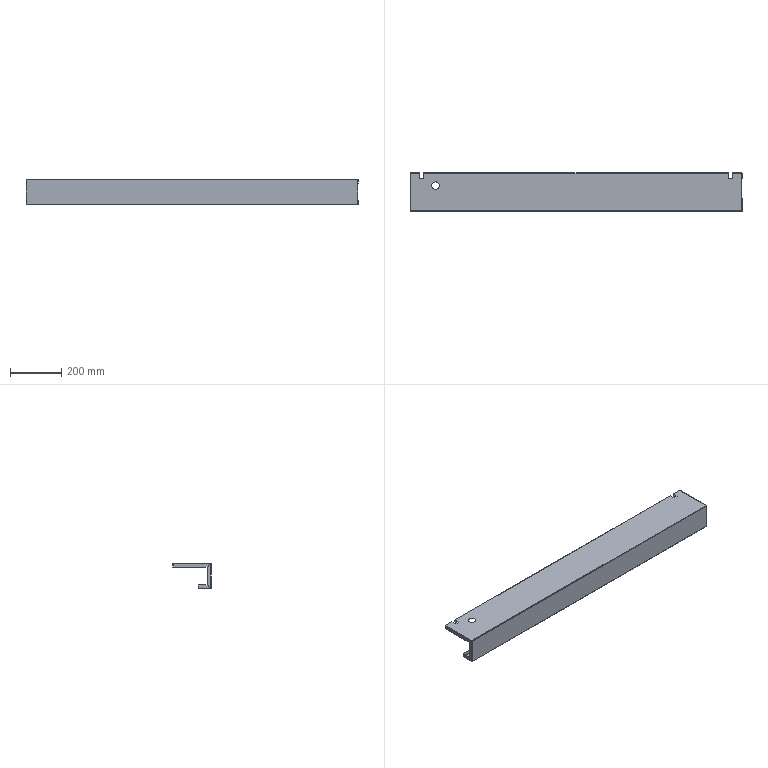Part | SolidWorks | features EdgeFlange 3, ICE 2, FlatPattern 1, SMBaseFlange 1, SheetMetal 1 | 1 solid | 112 faces | box 1298 x 148.8 x 100 mm | volume 507645 mm3 | plane 70 | cylinder 26 | spline 16 | commonest cylinder face diameters 0.9 x12 3.3 x12 30 x2